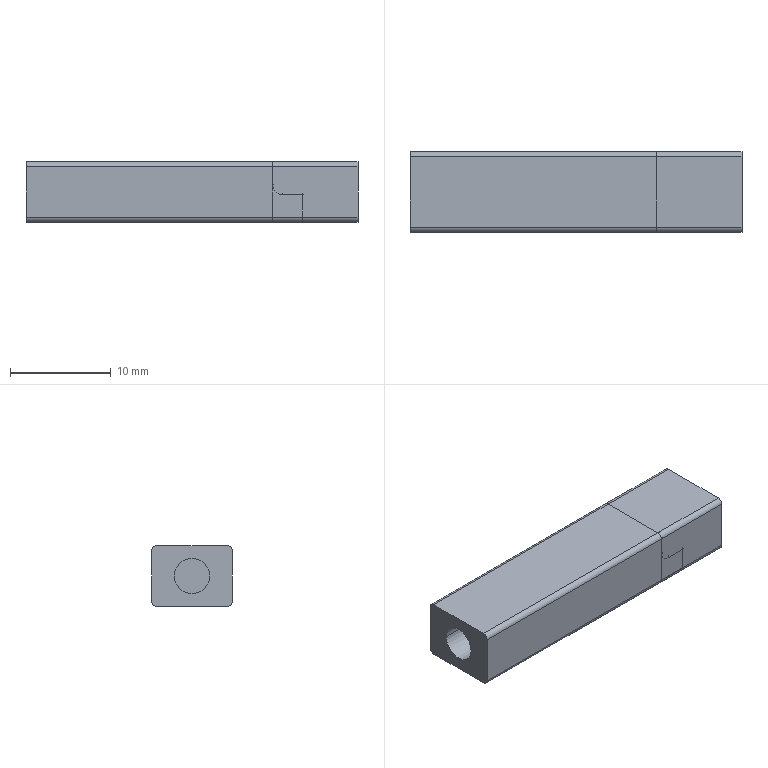NC program | NX | posted with a generic post | part box 33 x 8 x 6 mm
Whole program:
N10 G17 G21 G94 G90
(FLOOR_WALL , TOOL : D63)
N12 T01 M6
N14 G54
N16 G17 G0 G90 X-54. Y0. B0. C0. S6500 M3
N18 G43 Z30. H1
N20 Z3.
N22 G94 G1 Z0. F1250.
N24 X-51.
N26 X51.
N28 X54.
N30 Z3.
N32 G0 Z30.
N34 M5
(ZLEVEL_PROFILE , TOOL : D10)
N36 T09 M6
N38 G54
N40 G17 G0 G90 X9.367 Y9.1 B0. C0. S9500 M3
N42 G43 Z30. H9
N44 Z1.5
N46 G94 G1 X17.054 Z1.097 F1000.
N48 X18.398 Y8.766 Z1.025
N50 X19.604 Y8.084 Z0.952
N52 X20.584 Y7.104 Z0.879
N54 X21.266 Y5.898 Z0.807
N56 X21.6 Y4.554 Z0.734
N58 Y-4.554 Z0.257
N60 X21.266 Y-5.898 Z0.184
N62 X20.584 Y-7.104 Z0.112
N64 X19.604 Y-8.084 Z0.039
N66 X18.398 Y-8.766 Z-0.034
N68 X17.054 Y-9.1 Z-0.106
N70 X0. Z-1.
N72 X-16.5 F3000.
N74 G2 X-21.6 Y-4. R5.1
N76 G1 Y4.
N78 G2 X-16.5 Y9.1 R5.1
N80 G1 X16.5
N82 G2 X21.6 Y4. R5.1
N84 G1 Y-4.
N86 G2 X16.5 Y-9.1 R5.1
N88 G1 X0.
N90 X-16.258 Z-1.284
N92 X-16.645 Y-9.098 Z-1.291
N94 X-17.031 Y-9.072 Z-1.297
N96 X-17.414 Y-9.017 Z-1.304
N98 X-17.792 Y-8.934 Z-1.311
N100 X-18.162 Y-8.821 Z-1.318
N102 X-18.523 Y-8.681 Z-1.324
N104 X-18.872 Y-8.515 Z-1.331
N106 X-19.208 Y-8.322 Z-1.338
N108 X-19.528 Y-8.104 Z-1.345
N110 X-19.83 Y-7.862 Z-1.351
N112 X-20.114 Y-7.599 Z-1.358
N114 X-20.376 Y-7.314 Z-1.365
N116 X-20.616 Y-7.011 Z-1.372
N118 X-20.833 Y-6.69 Z-1.378
N120 X-21.024 Y-6.354 Z-1.385
N122 X-21.19 Y-6.004 Z-1.392
N124 X-21.328 Y-5.643 Z-1.399
N126 X-21.439 Y-5.272 Z-1.405
N128 X-21.521 Y-4.894 Z-1.412
N130 X-21.574 Y-4.51 Z-1.419
N132 X-21.598 Y-4.124 Z-1.426
N134 X-21.6 Y-3.737 Z-1.432
N136 Y3.618 Z-1.561
N138 Y4.005 Z-1.568
N140 X-21.585 Y4.392 Z-1.574
N142 X-21.541 Y4.776 Z-1.581
N144 X-21.467 Y5.156 Z-1.588
N146 X-21.365 Y5.529 Z-1.595
N148 X-21.235 Y5.894 Z-1.601
N150 X-21.078 Y6.247 Z-1.608
N152 X-20.894 Y6.588 Z-1.615
N154 X-20.686 Y6.914 Z-1.622
N156 X-20.453 Y7.223 Z-1.628
N158 X-20.197 Y7.513 Z-1.635
N160 X-19.92 Y7.784 Z-1.642
N162 X-19.623 Y8.032 Z-1.649
N164 X-19.308 Y8.257 Z-1.655
N166 X-18.977 Y8.458 Z-1.662
N168 X-18.632 Y8.633 Z-1.669
N170 X-18.275 Y8.781 Z-1.676
N172 X-17.907 Y8.902 Z-1.682
N174 X-17.531 Y8.995 Z-1.689
N176 X-17.15 Y9.058 Z-1.696
N178 X-16.764 Y9.093 Z-1.703
N180 X-16.377 Y9.1 Z-1.709
N182 X-15.99 Z-1.716
N184 X-0.119 Z-1.993
N186 X0.268 Z-2.
N188 X16.5
N190 G2 X21.6 Y4. R5.1
N192 G1 Y-4.
N194 G2 X16.5 Y-9.1 R5.1
N196 G1 X0.
N198 X-16.258 Z-2.284
N200 X-16.645 Y-9.098 Z-2.291
N202 X-17.031 Y-9.072 Z-2.297
N204 X-17.414 Y-9.017 Z-2.304
N206 X-17.792 Y-8.934 Z-2.311
N208 X-18.162 Y-8.821 Z-2.318
N210 X-18.523 Y-8.681 Z-2.324
N212 X-18.872 Y-8.515 Z-2.331
N214 X-19.208 Y-8.322 Z-2.338
N216 X-19.528 Y-8.104 Z-2.345
N218 X-19.83 Y-7.862 Z-2.351
N220 X-20.114 Y-7.599 Z-2.358
N222 X-20.376 Y-7.314 Z-2.365
N224 X-20.616 Y-7.011 Z-2.372
N226 X-20.833 Y-6.69 Z-2.378
N228 X-21.024 Y-6.354 Z-2.385
N230 X-21.19 Y-6.004 Z-2.392
N232 X-21.328 Y-5.643 Z-2.399
N234 X-21.439 Y-5.272 Z-2.405
N236 X-21.521 Y-4.894 Z-2.412
N238 X-21.574 Y-4.51 Z-2.419
N240 X-21.598 Y-4.124 Z-2.426
N242 X-21.6 Y-3.737 Z-2.432
N244 Y3.618 Z-2.561
N246 Y4.005 Z-2.568
N248 X-21.585 Y4.392 Z-2.574
N250 X-21.541 Y4.776 Z-2.581
N252 X-21.467 Y5.156 Z-2.588
N254 X-21.365 Y5.529 Z-2.595
N256 X-21.235 Y5.894 Z-2.601
N258 X-21.078 Y6.247 Z-2.608
N260 X-20.894 Y6.588 Z-2.615
N262 X-20.686 Y6.914 Z-2.622
N264 X-20.453 Y7.223 Z-2.628
N266 X-20.197 Y7.513 Z-2.635
N268 X-19.92 Y7.784 Z-2.642
N270 X-19.623 Y8.032 Z-2.649
N272 X-19.308 Y8.257 Z-2.655
N274 X-18.977 Y8.458 Z-2.662
N276 X-18.632 Y8.633 Z-2.669
N278 X-18.275 Y8.781 Z-2.676
N280 X-17.907 Y8.902 Z-2.682
N282 X-17.531 Y8.995 Z-2.689
N284 X-17.15 Y9.058 Z-2.696
N286 X-16.764 Y9.093 Z-2.703
N288 X-16.377 Y9.1 Z-2.709
N290 X-15.99 Z-2.716
N292 X-0.119 Z-2.993
N294 X0.268 Z-3.
N296 X16.5
N298 G2 X21.6 Y4. R5.1
N300 G1 Y-4.
N302 G2 X16.5 Y-9.1 R5.1
N304 G1 X0.
N306 X-16.258 Z-3.284
N308 X-16.645 Y-9.098 Z-3.291
N310 X-17.031 Y-9.072 Z-3.297
N312 X-17.414 Y-9.017 Z-3.304
N314 X-17.792 Y-8.934 Z-3.311
N316 X-18.162 Y-8.821 Z-3.318
N318 X-18.523 Y-8.681 Z-3.324
N320 X-18.872 Y-8.515 Z-3.331
N322 X-19.208 Y-8.322 Z-3.338
N324 X-19.528 Y-8.104 Z-3.345
N326 X-19.83 Y-7.862 Z-3.351
N328 X-20.114 Y-7.599 Z-3.358
N330 X-20.376 Y-7.314 Z-3.365
N332 X-20.616 Y-7.011 Z-3.372
N334 X-20.833 Y-6.69 Z-3.378
N336 X-21.024 Y-6.354 Z-3.385
N338 X-21.19 Y-6.004 Z-3.392
N340 X-21.328 Y-5.643 Z-3.399
N342 X-21.439 Y-5.272 Z-3.405
N344 X-21.521 Y-4.894 Z-3.412
N346 X-21.574 Y-4.51 Z-3.419
N348 X-21.598 Y-4.124 Z-3.426
N350 X-21.6 Y-3.737 Z-3.432
N352 Y3.618 Z-3.561
N354 Y4.005 Z-3.568
N356 X-21.585 Y4.392 Z-3.574
N358 X-21.541 Y4.776 Z-3.581
N360 X-21.467 Y5.156 Z-3.588
N362 X-21.365 Y5.529 Z-3.595
N364 X-21.235 Y5.894 Z-3.601
N366 X-21.078 Y6.247 Z-3.608
N368 X-20.894 Y6.588 Z-3.615
N370 X-20.686 Y6.914 Z-3.622
N372 X-20.453 Y7.223 Z-3.628
N374 X-20.197 Y7.513 Z-3.635
N376 X-19.92 Y7.784 Z-3.642
N378 X-19.623 Y8.032 Z-3.649
N380 X-19.308 Y8.257 Z-3.655
N382 X-18.977 Y8.458 Z-3.662
N384 X-18.632 Y8.633 Z-3.669
N386 X-18.275 Y8.781 Z-3.676
N388 X-17.907 Y8.902 Z-3.682
N390 X-17.531 Y8.995 Z-3.689
N392 X-17.15 Y9.058 Z-3.696
N394 X-16.764 Y9.093 Z-3.703
N396 X-16.377 Y9.1 Z-3.709
N398 X-15.99 Z-3.716
N400 X-0.119 Z-3.993
N402 X0.268 Z-4.
N404 X16.5
N406 G2 X21.6 Y4. R5.1
N408 G1 Y-4.
N410 G2 X16.5 Y-9.1 R5.1
N412 G1 X0.
N414 X-16.258 Z-4.284
N416 X-16.645 Y-9.098 Z-4.291
N418 X-17.031 Y-9.072 Z-4.297
N420 X-17.414 Y-9.017 Z-4.304
N422 X-17.792 Y-8.934 Z-4.311
N424 X-18.162 Y-8.821 Z-4.318
N426 X-18.523 Y-8.681 Z-4.324
N428 X-18.872 Y-8.515 Z-4.331
N430 X-19.208 Y-8.322 Z-4.338
N432 X-19.528 Y-8.104 Z-4.345
N434 X-19.83 Y-7.862 Z-4.351
N436 X-20.114 Y-7.599 Z-4.358
N438 X-20.376 Y-7.314 Z-4.365
N440 X-20.616 Y-7.011 Z-4.372
N442 X-20.833 Y-6.69 Z-4.378
N444 X-21.024 Y-6.354 Z-4.385
N446 X-21.19 Y-6.004 Z-4.392
N448 X-21.328 Y-5.643 Z-4.399
N450 X-21.439 Y-5.272 Z-4.405
N452 X-21.521 Y-4.894 Z-4.412
N454 X-21.574 Y-4.51 Z-4.419
N456 X-21.598 Y-4.124 Z-4.426
N458 X-21.6 Y-3.737 Z-4.432
N460 Y3.618 Z-4.561
N462 Y4.005 Z-4.568
N464 X-21.585 Y4.392 Z-4.574
N466 X-21.541 Y4.776 Z-4.581
N468 X-21.467 Y5.156 Z-4.588
N470 X-21.365 Y5.529 Z-4.595
N472 X-21.235 Y5.894 Z-4.601
N474 X-21.078 Y6.247 Z-4.608
N476 X-20.894 Y6.588 Z-4.615
N478 X-20.686 Y6.914 Z-4.622
N480 X-20.453 Y7.223 Z-4.628
N482 X-20.197 Y7.513 Z-4.635
N484 X-19.92 Y7.784 Z-4.642
N486 X-19.623 Y8.032 Z-4.649
N488 X-19.308 Y8.257 Z-4.655
N490 X-18.977 Y8.458 Z-4.662
N492 X-18.632 Y8.633 Z-4.669
N494 X-18.275 Y8.781 Z-4.676
N496 X-17.907 Y8.902 Z-4.682
N498 X-17.531 Y8.995 Z-4.689
N500 X-17.15 Y9.058 Z-4.696
N502 X-16.764 Y9.093 Z-4.703
N504 X-16.377 Y9.1 Z-4.709
N506 X-15.99 Z-4.716
N508 X-0.119 Z-4.993
N510 X0.268 Z-5.
N512 X16.5
N514 G2 X21.6 Y4. R5.1
N516 G1 Y-4.
N518 G2 X16.5 Y-9.1 R5.1
N520 G1 X0.
N522 X-16.258 Z-5.284
N524 X-16.645 Y-9.098 Z-5.291
N526 X-17.031 Y-9.072 Z-5.297
N528 X-17.414 Y-9.017 Z-5.304
N530 X-17.792 Y-8.934 Z-5.311
N532 X-18.162 Y-8.821 Z-5.318
N534 X-18.523 Y-8.681 Z-5.324
N536 X-18.872 Y-8.515 Z-5.331
N538 X-19.208 Y-8.322 Z-5.338
N540 X-19.528 Y-8.104 Z-5.345
N542 X-19.83 Y-7.862 Z-5.351
N544 X-20.114 Y-7.599 Z-5.358
N546 X-20.376 Y-7.314 Z-5.365
N548 X-20.616 Y-7.011 Z-5.372
N550 X-20.833 Y-6.69 Z-5.378
N552 X-21.024 Y-6.354 Z-5.385
N554 X-21.19 Y-6.004 Z-5.392
N556 X-21.328 Y-5.643 Z-5.399
N558 X-21.439 Y-5.272 Z-5.405
N560 X-21.521 Y-4.894 Z-5.412
N562 X-21.574 Y-4.51 Z-5.419
N564 X-21.598 Y-4.124 Z-5.426
N566 X-21.6 Y-3.737 Z-5.432
N568 Y3.618 Z-5.561
N570 Y4.005 Z-5.568
N572 X-21.585 Y4.392 Z-5.574
N574 X-21.541 Y4.776 Z-5.581
N576 X-21.467 Y5.156 Z-5.588
N578 X-21.365 Y5.529 Z-5.595
N580 X-21.235 Y5.894 Z-5.601
N582 X-21.078 Y6.247 Z-5.608
N584 X-20.894 Y6.588 Z-5.615
N586 X-20.686 Y6.914 Z-5.622
N588 X-20.453 Y7.223 Z-5.628
N590 X-20.197 Y7.513 Z-5.635
N592 X-19.92 Y7.784 Z-5.642
N594 X-19.623 Y8.032 Z-5.649
N596 X-19.308 Y8.257 Z-5.655
N598 X-18.977 Y8.458 Z-5.662
N600 X-18.632 Y8.633 Z-5.669
N602 X-18.275 Y8.781 Z-5.676
N604 X-17.907 Y8.902 Z-5.682
N606 X-17.531 Y8.995 Z-5.689
N608 X-17.15 Y9.058 Z-5.696
N610 X-16.764 Y9.093 Z-5.703
N612 X-16.377 Y9.1 Z-5.709
N614 X-15.99 Z-5.716
N616 X-0.119 Z-5.993
N618 X0.268 Z-6.
N620 X16.5
N622 G2 X21.6 Y4. R5.1
N624 G1 Y-4.
N626 G2 X16.5 Y-9.1 R5.1
N628 G1 X-16.5
N630 G2 X-21.6 Y-4. R5.1
N632 G1 Y4.
N634 G2 X-16.5 Y9.1 R5.1
N636 G1 X0.268
N638 Z-4.5
N640 G0 Z30.
N642 M5
(ZLEVEL_PROFILE_COPY_COPY , TOOL : D10JING)
N644 T10 M6
N646 G54
N648 G17 G0 G90 X18.122 Y-10.809 B0. C0. S9500 M3
N650 G43 Z30. H10
N652 Z-4.5
N654 G94 G1 Z-6. F1000.
N656 X17.366 Y-9.5
N658 G3 X16.5 Y-9. R1.
N660 G1 X-16.5 F1200.
N662 G2 X-21.5 Y-4. R5.
N664 G1 Y4.
N666 G2 X-16.5 Y9. R5.
N668 G1 X16.5
N670 G2 X21.5 Y4. R5.
N672 G1 Y-4.
N674 G2 X16.5 Y-9. R5.
N676 G3 X15.634 Y-9.5 R1.
N678 G1 X14.768 Y-11.
N680 Z-4.5
N682 G0 Z30.
N684 M5
(ZLEVEL_PROFILE_COPY_1 , TOOL : D6R0.5)
N686 T08 M6
N688 G54
N690 G17 G0 G90 X20.681 Y-7.206 B0. C0. S9500 M3
N692 G43 Z30. H8
N694 Z1.483
N696 G94 G1 Z-0.017 F1000.
N698 X20.298 Y-6.447
N700 G3 X19.796 Y-6.119 R0.6
N702 G1 X19.512 Y-6.103 F3000.
N704 X17.095 Y-6.139
N706 X16.5 Y-6.185
N708 X-16.5
N710 X-19.512 Y-6.103
N712 X-19.796 Y-6.119
N714 X-19.798 Y-6.165 Z-0.028
N716 X-19.8 Y-6.192 Z-0.039
N718 X-16.75 Y-6.251
N720 X-16.5 Y-6.276
N722 X16.5
N724 X17.095 Y-6.225
N726 X19.8 Y-6.193
N728 Y-6.239 Z-0.052
N730 Y-6.268 Z-0.066
N732 G3 X16.5 Y-6.358 R33.279
N734 G1 X-16.5
N736 G3 X-19.8 Y-6.263 R44.502
N738 G1 Y-6.312 Z-0.083
N740 Y-6.343 Z-0.1
N742 G2 X-16.5 Y-6.435 R39.091
N744 G1 X16.5
N746 G2 X19.8 Y-6.348 R37.595
N748 G1 Y-6.391 Z-0.12
N750 Y-6.42 Z-0.141
N752 G3 X16.5 Y-6.512 R36.842
N754 G1 X-16.5
N756 G3 X-19.8 Y-6.415 R38.811
N758 G1 Y-6.46 Z-0.166
N760 Y-6.5 Z-0.191
N762 G2 X-16.5 Y-6.587 R41.049
N764 G1 X16.5
N766 G2 X19.8 Y-6.504 R37.094
N768 G1 Y-6.547 Z-0.22
N770 Y-6.583 Z-0.249
N772 G3 X16.5 Y-6.66 R43.627
N774 G1 X-16.5
N776 G3 X-19.8 Y-6.581 R45.358
N778 G1 Y-6.627 Z-0.282
N780 Y-6.672 Z-0.315
N782 G2 X-16.5 Y-6.729 R56.408
N784 G1 X16.5
N786 G2 X19.8 Y-6.672 R56.54
N788 G1 Y-6.702 Z-0.352
N790 Y-6.726 Z-0.389
N792 G3 X16.5 Y-6.792 R53.301
N794 G1 X-16.5
N796 G3 X-19.8 Y-6.727 R51.414
N798 G1 Y-6.763 Z-0.43
N800 Y-6.788 Z-0.47
N802 G2 X-16.5 Y-6.848 R53.735
N804 G1 X16.5
N806 G2 X19.8 Y-6.785 R58.206
N808 G1 Y-6.818 Z-0.513
N810 Y-6.846 Z-0.556
N812 G3 X16.5 Y-6.896 R72.254
N814 G1 X-16.5
N816 G3 X-19.8 Y-6.849 R63.779
N818 G1 Y-6.873 Z-0.602
N820 Y-6.898 Z-0.648
N822 G2 X-16.5 Y-6.936 R83.782
N824 G1 X16.5
N826 G2 X19.8 Y-6.895 R109.452
N828 G1 Y-6.92 Z-0.695
N830 Y-6.938 Z-0.743
N832 G3 X16.5 Y-6.966 R139.65
N834 G1 X-16.5
N836 G3 X-19.8 Y-6.94 R119.589
N838 G1 Y-6.958 Z-0.792
N840 Y-6.97 Z-0.84
N842 X-17.095 Y-6.976
N844 X-16.5 Y-6.987
N846 X16.5
N848 G2 X19.8 Y-6.97 R203.121
N850 G1 Y-6.984 Z-0.89
N852 Y-6.996 Z-0.94
N854 X16.75
N856 X16.5 Y-6.998
N858 X-16.5
N860 X-16.75 Y-6.996
N862 X-19.8
N864 Y-6.997 Z-1.04
N866 X19.8
N868 Z-1.14
N870 X-19.8
N872 Z-1.23
N874 X19.8
N876 Z-1.32
N878 X-19.8
N880 Z-1.41
N882 X19.8
N884 Z-1.5
N886 X-19.8
N888 G3 X-20.32 Y-7.297 R0.6
N890 G1 X-20.773 Y-8.083
N892 Z0.
N894 G0 Z30.
N896 X-20.681 Y7.206
N898 Z1.483
N900 G1 Z-0.017 F1000.
N902 X-20.298 Y6.447
N904 G3 X-19.796 Y6.119 R0.6
N906 G1 X-19.512 Y6.103 F3000.
N908 X-17.095 Y6.139
N910 X-16.5 Y6.185
N912 X16.5
N914 X19.512 Y6.103
N916 X19.796 Y6.119
N918 X19.798 Y6.165 Z-0.028
N920 X19.8 Y6.192 Z-0.039
N922 X16.75 Y6.251
N924 X16.5 Y6.276
N926 X-16.5
N928 X-17.095 Y6.225
N930 X-19.8 Y6.193
N932 Y6.239 Z-0.052
N934 Y6.268 Z-0.066
N936 G3 X-16.5 Y6.358 R33.28
N938 G1 X8.002
N940 X16.5
N942 G3 X19.8 Y6.263 R44.5
N944 G1 Y6.306 Z-0.083
N946 Y6.343 Z-0.1
N948 G2 X16.5 Y6.435 R39.089
N950 G1 X-16.5
N952 G2 X-19.8 Y6.348 R37.596
N954 G1 Y6.391 Z-0.12
N956 Y6.42 Z-0.141
N958 G3 X-16.5 Y6.512 R36.843
N960 G1 X8.002
N962 X16.5
N964 G3 X19.8 Y6.415 R38.809
N966 G1 Y6.46 Z-0.166
N968 Y6.5 Z-0.191
N970 G2 X16.5 Y6.587 R41.047
N972 G1 X-16.5
N974 G2 X-19.8 Y6.504 R37.096
N976 G1 Y6.547 Z-0.22
N978 Y6.583 Z-0.249
N980 G3 X-16.5 Y6.66 R43.629
N982 G1 X8.002
N984 X16.5
N986 G3 X19.8 Y6.581 R45.356
N988 G1 Y6.627 Z-0.282
N990 Y6.672 Z-0.315
N992 G2 X16.5 Y6.729 R56.406
N994 G1 X-16.5
N996 G2 X-19.8 Y6.672 R56.542
N998 G1 Y6.702 Z-0.352
N1000 Y6.726 Z-0.389
N1002 G3 X-16.5 Y6.792 R53.303
N1004 G1 X8.002
N1006 X16.5
N1008 G3 X19.8 Y6.727 R51.412
N1010 G1 Y6.763 Z-0.43
N1012 Y6.788 Z-0.47
N1014 G2 X16.5 Y6.848 R53.733
N1016 G1 X-16.5
N1018 G2 X-19.8 Y6.785 R58.209
N1020 G1 Y6.818 Z-0.513
N1022 Y6.846 Z-0.556
N1024 G3 X-16.5 Y6.896 R72.257
N1026 G1 X16.5
N1028 G3 X19.8 Y6.849 R63.775
N1030 G1 Y6.873 Z-0.602
N1032 Y6.898 Z-0.648
N1034 G2 X16.5 Y6.936 R83.778
N1036 G1 X-16.5
N1038 G2 X-19.8 Y6.895 R109.457
N1040 G1 Y6.915 Z-0.695
N1042 Y6.938 Z-0.743
N1044 G3 X-16.5 Y6.966 R139.657
N1046 G1 X8.002
N1048 X16.5
N1050 G3 X19.8 Y6.94 R112.667
N1052 G1 Y6.956 Z-0.792
N1054 Y6.97 Z-0.84
N1056 X17.095 Y6.976
N1058 X16.5 Y6.987
N1060 X-16.5
N1062 G2 X-19.8 Y6.97 R203.133
N1064 G1 Y6.988 Z-0.89
N1066 Y6.996 Z-0.94
N1068 X-16.5 Y6.998
N1070 X16.5
N1072 X19.8 Y6.996
N1074 X19.799 Y6.999 Z-1.04
N1076 X-19.799
N1078 Z-1.14
N1080 X19.799
N1082 Z-1.23
N1084 X-19.799
N1086 Z-1.32
N1088 X19.799
N1090 Z-1.41
N1092 X-19.799
N1094 Z-1.5
N1096 X19.799
N1098 G3 X20.319 Y7.299 R0.6
N1100 G1 X20.772 Y8.085
N1102 Z0.
N1104 G0 Z30.
N1106 M5
N1108 M2